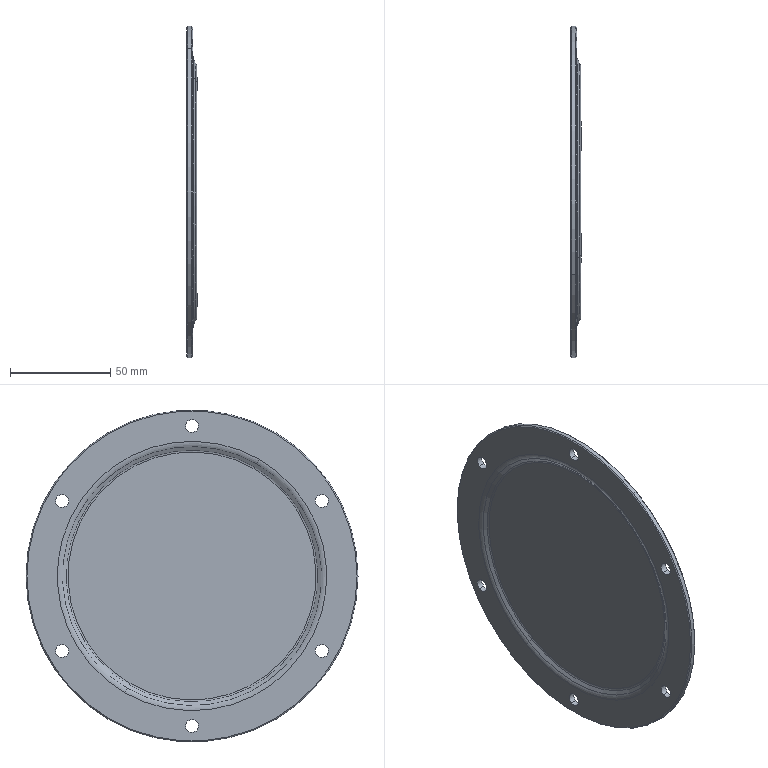Part | SolidWorks | features BaseBody 1 | 1 solid | 34 faces | box 5 x 166 x 166 mm | volume 64748 mm3 | cylinder 14 | cone 8 | torus 8 | plane 4 | commonest cylinder face diameters 6.5 x12 166 x2
STEP:
#1=CARTESIAN_POINT('',(330.,-41.5,71.88));
#2=VERTEX_POINT('',#1);
#3=CARTESIAN_POINT('',(330.,41.5,-71.88));
#4=VERTEX_POINT('',#3);
#5=CARTESIAN_POINT('',(330.,0.,0.));
#6=DIRECTION('',(-1.,0.,0.));
#7=DIRECTION('',(0.,-0.5,0.866));
#8=AXIS2_PLACEMENT_3D('',#5,#6,#7);
#9=CIRCLE('',#8,83.);
#10=EDGE_CURVE('',#2,#4,#9,.T.);
#11=ORIENTED_EDGE('',*,*,#10,.T.);
#12=CARTESIAN_POINT('',(328.,41.5,-71.88));
#13=VERTEX_POINT('',#12);
#14=CARTESIAN_POINT('',(330.,41.5,-71.88));
#15=DIRECTION('',(-1.,0.,0.));
#16=VECTOR('',#15,1000.);
#17=LINE('',#14,#16);
#18=EDGE_CURVE('',#4,#13,#17,.T.);
#19=ORIENTED_EDGE('',*,*,#18,.T.);
#20=CARTESIAN_POINT('',(328.,-41.5,71.88));
#21=VERTEX_POINT('',#20);
#22=CARTESIAN_POINT('',(328.,0.,0.));
#23=DIRECTION('',(1.,0.,0.));
#24=DIRECTION('',(0.,0.5,-0.866));
#25=AXIS2_PLACEMENT_3D('',#22,#23,#24);
#26=CIRCLE('',#25,83.);
#27=EDGE_CURVE('',#13,#21,#26,.T.);
#28=ORIENTED_EDGE('',*,*,#27,.T.);
#29=CARTESIAN_POINT('',(330.,-41.5,71.88));
#30=DIRECTION('',(-1.,0.,0.));
#31=VECTOR('',#30,1000.);
#32=LINE('',#29,#31);
#33=EDGE_CURVE('',#2,#21,#32,.T.);
#34=ORIENTED_EDGE('',*,*,#33,.F.);
#35=EDGE_LOOP('',(#11,#19,#28,#34));
#36=FACE_OUTER_BOUND('',#35,.T.);
#37=CARTESIAN_POINT('',(330.,0.,0.));
#38=DIRECTION('',(-1.,0.,0.));
#39=DIRECTION('',(0.,-0.5,0.866));
#40=AXIS2_PLACEMENT_3D('',#37,#38,#39);
#41=CYLINDRICAL_SURFACE('',#40,83.);
#42=ADVANCED_FACE('',(#36),#41,.T.);
#43=CARTESIAN_POINT('',(331.83,-32.25,55.859));
#44=VERTEX_POINT('',#43);
#45=CARTESIAN_POINT('',(331.83,32.25,-55.859));
#46=VERTEX_POINT('',#45);
#47=CARTESIAN_POINT('',(331.83,0.,0.));
#48=DIRECTION('',(-1.,0.,0.));
#49=DIRECTION('',(0.,0.5,-0.866));
#50=AXIS2_PLACEMENT_3D('',#47,#48,#49);
#51=CIRCLE('',#50,64.5);
#52=EDGE_CURVE('',#44,#46,#51,.T.);
#53=ORIENTED_EDGE('',*,*,#52,.T.);
#54=CARTESIAN_POINT('',(330.768,33.17,-57.452));
#55=VERTEX_POINT('',#54);
#56=CARTESIAN_POINT('',(368.069,0.866,-1.5));
#57=DIRECTION('',(-0.5,0.433,-0.75));
#58=VECTOR('',#57,1000.);
#59=LINE('',#56,#58);
#60=EDGE_CURVE('',#46,#55,#59,.T.);
#61=ORIENTED_EDGE('',*,*,#60,.T.);
#62=CARTESIAN_POINT('',(330.768,-33.17,57.452));
#63=VERTEX_POINT('',#62);
#64=CARTESIAN_POINT('',(330.768,0.,0.));
#65=DIRECTION('',(1.,0.,0.));
#66=DIRECTION('',(0.,0.5,-0.866));
#67=AXIS2_PLACEMENT_3D('',#64,#65,#66);
#68=CIRCLE('',#67,66.34);
#69=EDGE_CURVE('',#55,#63,#68,.T.);
#70=ORIENTED_EDGE('',*,*,#69,.T.);
#71=CARTESIAN_POINT('',(368.069,-0.866,1.5));
#72=DIRECTION('',(-0.5,-0.433,0.75));
#73=VECTOR('',#72,1000.);
#74=LINE('',#71,#73);
#75=EDGE_CURVE('',#44,#63,#74,.T.);
#76=ORIENTED_EDGE('',*,*,#75,.F.);
#77=EDGE_LOOP('',(#53,#61,#70,#76));
#78=FACE_OUTER_BOUND('',#77,.T.);
#79=CARTESIAN_POINT('',(368.069,0.,0.));
#80=DIRECTION('',(-1.,0.,0.));
#81=DIRECTION('',(0.,-0.5,0.866));
#82=AXIS2_PLACEMENT_3D('',#79,#80,#81);
#83=CONICAL_SURFACE('',#82,1.732,1.047);
#84=ADVANCED_FACE('',(#78),#83,.T.);
#85=CARTESIAN_POINT('',(329.232,-31.5,54.56));
#86=VERTEX_POINT('',#85);
#87=CARTESIAN_POINT('',(329.232,31.5,-54.56));
#88=VERTEX_POINT('',#87);
#89=CARTESIAN_POINT('',(329.232,0.,0.));
#90=DIRECTION('',(1.,0.,0.));
#91=DIRECTION('',(0.,0.5,-0.866));
#92=AXIS2_PLACEMENT_3D('',#89,#90,#91);
#93=CIRCLE('',#92,63.);
#94=EDGE_CURVE('',#86,#88,#93,.T.);
#95=ORIENTED_EDGE('',*,*,#94,.T.);
#96=CARTESIAN_POINT('',(328.17,32.42,-56.153));
#97=VERTEX_POINT('',#96);
#98=CARTESIAN_POINT('',(364.605,0.866,-1.5));
#99=DIRECTION('',(-0.5,0.433,-0.75));
#100=VECTOR('',#99,1000.);
#101=LINE('',#98,#100);
#102=EDGE_CURVE('',#88,#97,#101,.T.);
#103=ORIENTED_EDGE('',*,*,#102,.T.);
#104=CARTESIAN_POINT('',(328.17,-32.42,56.153));
#105=VERTEX_POINT('',#104);
#106=CARTESIAN_POINT('',(328.17,0.,0.));
#107=DIRECTION('',(-1.,0.,0.));
#108=DIRECTION('',(0.,0.5,-0.866));
#109=AXIS2_PLACEMENT_3D('',#106,#107,#108);
#110=CIRCLE('',#109,64.84);
#111=EDGE_CURVE('',#97,#105,#110,.T.);
#112=ORIENTED_EDGE('',*,*,#111,.T.);
#113=CARTESIAN_POINT('',(364.605,-0.866,1.5));
#114=DIRECTION('',(-0.5,-0.433,0.75));
#115=VECTOR('',#114,1000.);
#116=LINE('',#113,#115);
#117=EDGE_CURVE('',#86,#105,#116,.T.);
#118=ORIENTED_EDGE('',*,*,#117,.F.);
#119=EDGE_LOOP('',(#95,#103,#112,#118));
#120=FACE_OUTER_BOUND('',#119,.T.);
#121=CARTESIAN_POINT('',(364.605,0.,0.));
#122=DIRECTION('',(-1.,0.,0.));
#123=DIRECTION('',(0.,-0.5,0.866));
#124=AXIS2_PLACEMENT_3D('',#121,#122,#123);
#125=CONICAL_SURFACE('',#124,1.732,1.047);
#126=ADVANCED_FACE('',(#120),#125,.F.);
#127=ORIENTED_EDGE('',*,*,#52,.F.);
#128=CARTESIAN_POINT('',(332.5,-31.,53.694));
#129=VERTEX_POINT('',#128);
#130=CARTESIAN_POINT('',(327.5,-31.,53.694));
#131=DIRECTION('',(0.,0.866,0.5));
#132=DIRECTION('',(0.,-0.5,0.866));
#133=AXIS2_PLACEMENT_3D('',#130,#131,#132);
#134=CIRCLE('',#133,5.);
#135=EDGE_CURVE('',#44,#129,#134,.T.);
#136=ORIENTED_EDGE('',*,*,#135,.T.);
#137=CARTESIAN_POINT('',(332.5,31.,-53.694));
#138=VERTEX_POINT('',#137);
#139=CARTESIAN_POINT('',(332.5,0.,0.));
#140=DIRECTION('',(1.,0.,0.));
#141=DIRECTION('',(0.,-0.5,0.866));
#142=AXIS2_PLACEMENT_3D('',#139,#140,#141);
#143=CIRCLE('',#142,62.);
#144=EDGE_CURVE('',#138,#129,#143,.T.);
#145=ORIENTED_EDGE('',*,*,#144,.F.);
#146=CARTESIAN_POINT('',(327.5,31.,-53.694));
#147=DIRECTION('',(0.,-0.866,-0.5));
#148=DIRECTION('',(0.,0.5,-0.866));
#149=AXIS2_PLACEMENT_3D('',#146,#147,#148);
#150=CIRCLE('',#149,5.);
#151=EDGE_CURVE('',#46,#138,#150,.T.);
#152=ORIENTED_EDGE('',*,*,#151,.F.);
#153=EDGE_LOOP('',(#127,#136,#145,#152));
#154=FACE_OUTER_BOUND('',#153,.T.);
#155=CARTESIAN_POINT('',(327.5,0.,0.));
#156=DIRECTION('',(1.,0.,0.));
#157=DIRECTION('',(0.,0.5,-0.866));
#158=AXIS2_PLACEMENT_3D('',#155,#156,#157);
#159=TOROIDAL_SURFACE('',#158,62.,5.);
#160=ADVANCED_FACE('',(#154),#159,.T.);
#161=CARTESIAN_POINT('',(327.5,33.67,-58.318));
#162=VERTEX_POINT('',#161);
#163=CARTESIAN_POINT('',(327.5,-33.67,58.318));
#164=VERTEX_POINT('',#163);
#165=CARTESIAN_POINT('',(327.5,0.,0.));
#166=DIRECTION('',(1.,0.,0.));
#167=DIRECTION('',(0.,0.5,-0.866));
#168=AXIS2_PLACEMENT_3D('',#165,#166,#167);
#169=CIRCLE('',#168,67.34);
#170=EDGE_CURVE('',#162,#164,#169,.T.);
#171=ORIENTED_EDGE('',*,*,#170,.F.);
#172=CARTESIAN_POINT('',(332.5,33.67,-58.318));
#173=DIRECTION('',(0.,0.866,0.5));
#174=DIRECTION('',(0.,-0.5,0.866));
#175=AXIS2_PLACEMENT_3D('',#172,#173,#174);
#176=CIRCLE('',#175,5.);
#177=EDGE_CURVE('',#162,#97,#176,.T.);
#178=ORIENTED_EDGE('',*,*,#177,.T.);
#179=CARTESIAN_POINT('',(328.17,0.,0.));
#180=DIRECTION('',(-1.,0.,0.));
#181=DIRECTION('',(0.,0.5,-0.866));
#182=AXIS2_PLACEMENT_3D('',#179,#180,#181);
#183=CIRCLE('',#182,64.84);
#184=EDGE_CURVE('',#105,#97,#183,.T.);
#185=ORIENTED_EDGE('',*,*,#184,.F.);
#186=CARTESIAN_POINT('',(332.5,-33.67,58.318));
#187=DIRECTION('',(0.,-0.866,-0.5));
#188=DIRECTION('',(0.,0.5,-0.866));
#189=AXIS2_PLACEMENT_3D('',#186,#187,#188);
#190=CIRCLE('',#189,5.);
#191=EDGE_CURVE('',#164,#105,#190,.T.);
#192=ORIENTED_EDGE('',*,*,#191,.F.);
#193=EDGE_LOOP('',(#171,#178,#185,#192));
#194=FACE_OUTER_BOUND('',#193,.T.);
#195=CARTESIAN_POINT('',(332.5,0.,0.));
#196=DIRECTION('',(-1.,0.,0.));
#197=DIRECTION('',(0.,-0.5,0.866));
#198=AXIS2_PLACEMENT_3D('',#195,#196,#197);
#199=TOROIDAL_SURFACE('',#198,67.34,5.);
#200=ADVANCED_FACE('',(#194),#199,.T.);
#201=CARTESIAN_POINT('',(330.768,0.,0.));
#202=DIRECTION('',(1.,0.,0.));
#203=DIRECTION('',(0.,0.5,-0.866));
#204=AXIS2_PLACEMENT_3D('',#201,#202,#203);
#205=CIRCLE('',#204,66.34);
#206=EDGE_CURVE('',#63,#55,#205,.T.);
#207=ORIENTED_EDGE('',*,*,#206,.F.);
#208=CARTESIAN_POINT('',(330.5,-33.67,58.318));
#209=VERTEX_POINT('',#208);
#210=CARTESIAN_POINT('',(332.5,-33.67,58.318));
#211=DIRECTION('',(0.,0.866,0.5));
#212=DIRECTION('',(0.,-0.5,0.866));
#213=AXIS2_PLACEMENT_3D('',#210,#211,#212);
#214=CIRCLE('',#213,2.);
#215=EDGE_CURVE('',#63,#209,#214,.T.);
#216=ORIENTED_EDGE('',*,*,#215,.T.);
#217=CARTESIAN_POINT('',(330.5,33.67,-58.318));
#218=VERTEX_POINT('',#217);
#219=CARTESIAN_POINT('',(330.5,0.,0.));
#220=DIRECTION('',(-1.,0.,0.));
#221=DIRECTION('',(0.,-0.5,0.866));
#222=AXIS2_PLACEMENT_3D('',#219,#220,#221);
#223=CIRCLE('',#222,67.34);
#224=EDGE_CURVE('',#218,#209,#223,.T.);
#225=ORIENTED_EDGE('',*,*,#224,.F.);
#226=CARTESIAN_POINT('',(332.5,33.67,-58.318));
#227=DIRECTION('',(0.,-0.866,-0.5));
#228=DIRECTION('',(0.,0.5,-0.866));
#229=AXIS2_PLACEMENT_3D('',#226,#227,#228);
#230=CIRCLE('',#229,2.);
#231=EDGE_CURVE('',#55,#218,#230,.T.);
#232=ORIENTED_EDGE('',*,*,#231,.F.);
#233=EDGE_LOOP('',(#207,#216,#225,#232));
#234=FACE_OUTER_BOUND('',#233,.T.);
#235=CARTESIAN_POINT('',(332.5,0.,0.));
#236=DIRECTION('',(1.,0.,0.));
#237=DIRECTION('',(0.,0.5,-0.866));
#238=AXIS2_PLACEMENT_3D('',#235,#236,#237);
#239=TOROIDAL_SURFACE('',#238,67.34,2.);
#240=ADVANCED_FACE('',(#234),#239,.F.);
#241=CARTESIAN_POINT('',(329.5,31.,-53.694));
#242=VERTEX_POINT('',#241);
#243=CARTESIAN_POINT('',(329.5,-31.,53.694));
#244=VERTEX_POINT('',#243);
#245=CARTESIAN_POINT('',(329.5,0.,0.));
#246=DIRECTION('',(-1.,0.,0.));
#247=DIRECTION('',(0.,0.5,-0.866));
#248=AXIS2_PLACEMENT_3D('',#245,#246,#247);
#249=CIRCLE('',#248,62.);
#250=EDGE_CURVE('',#242,#244,#249,.T.);
#251=ORIENTED_EDGE('',*,*,#250,.F.);
#252=CARTESIAN_POINT('',(327.5,31.,-53.694));
#253=DIRECTION('',(0.,0.866,0.5));
#254=DIRECTION('',(0.,-0.5,0.866));
#255=AXIS2_PLACEMENT_3D('',#252,#253,#254);
#256=CIRCLE('',#255,2.);
#257=EDGE_CURVE('',#242,#88,#256,.T.);
#258=ORIENTED_EDGE('',*,*,#257,.T.);
#259=ORIENTED_EDGE('',*,*,#94,.F.);
#260=CARTESIAN_POINT('',(327.5,-31.,53.694));
#261=DIRECTION('',(0.,-0.866,-0.5));
#262=DIRECTION('',(0.,0.5,-0.866));
#263=AXIS2_PLACEMENT_3D('',#260,#261,#262);
#264=CIRCLE('',#263,2.);
#265=EDGE_CURVE('',#244,#86,#264,.T.);
#266=ORIENTED_EDGE('',*,*,#265,.F.);
#267=EDGE_LOOP('',(#251,#258,#259,#266));
#268=FACE_OUTER_BOUND('',#267,.T.);
#269=CARTESIAN_POINT('',(327.5,0.,0.));
#270=DIRECTION('',(-1.,0.,0.));
#271=DIRECTION('',(0.,-0.5,0.866));
#272=AXIS2_PLACEMENT_3D('',#269,#270,#271);
#273=TOROIDAL_SURFACE('',#272,62.,2.);
#274=ADVANCED_FACE('',(#268),#273,.F.);
#275=CARTESIAN_POINT('',(330.5,41.25,-71.447));
#276=VERTEX_POINT('',#275);
#277=CARTESIAN_POINT('',(330.5,-41.25,71.447));
#278=VERTEX_POINT('',#277);
#279=CARTESIAN_POINT('',(330.5,0.,0.));
#280=DIRECTION('',(1.,0.,0.));
#281=DIRECTION('',(0.,-0.5,0.866));
#282=AXIS2_PLACEMENT_3D('',#279,#280,#281);
#283=CIRCLE('',#282,82.5);
#284=EDGE_CURVE('',#276,#278,#283,.T.);
#285=ORIENTED_EDGE('',*,*,#284,.F.);
#286=CARTESIAN_POINT('',(412.,0.5,-0.866));
#287=DIRECTION('',(-0.7071,0.3536,-0.6124));
#288=VECTOR('',#287,1000.);
#289=LINE('',#286,#288);
#290=EDGE_CURVE('',#276,#4,#289,.T.);
#291=ORIENTED_EDGE('',*,*,#290,.T.);
#292=ORIENTED_EDGE('',*,*,#10,.F.);
#293=CARTESIAN_POINT('',(412.,-0.5,0.866));
#294=DIRECTION('',(-0.7071,-0.3536,0.6124));
#295=VECTOR('',#294,1000.);
#296=LINE('',#293,#295);
#297=EDGE_CURVE('',#278,#2,#296,.T.);
#298=ORIENTED_EDGE('',*,*,#297,.F.);
#299=EDGE_LOOP('',(#285,#291,#292,#298));
#300=FACE_OUTER_BOUND('',#299,.T.);
#301=CARTESIAN_POINT('',(412.,0.,0.));
#302=DIRECTION('',(-1.,0.,0.));
#303=DIRECTION('',(0.,-0.5,0.866));
#304=AXIS2_PLACEMENT_3D('',#301,#302,#303);
#305=CONICAL_SURFACE('',#304,1.,0.7854);
#306=ADVANCED_FACE('',(#300),#305,.T.);
#307=CARTESIAN_POINT('',(327.5,-41.25,71.447));
#308=VERTEX_POINT('',#307);
#309=CARTESIAN_POINT('',(327.5,41.25,-71.447));
#310=VERTEX_POINT('',#309);
#311=CARTESIAN_POINT('',(327.5,0.,0.));
#312=DIRECTION('',(-1.,0.,0.));
#313=DIRECTION('',(0.,0.5,-0.866));
#314=AXIS2_PLACEMENT_3D('',#311,#312,#313);
#315=CIRCLE('',#314,82.5);
#316=EDGE_CURVE('',#308,#310,#315,.T.);
#317=ORIENTED_EDGE('',*,*,#316,.F.);
#318=CARTESIAN_POINT('',(246.,-0.5,0.866));
#319=DIRECTION('',(0.7071,-0.3536,0.6124));
#320=VECTOR('',#319,1000.);
#321=LINE('',#318,#320);
#322=EDGE_CURVE('',#308,#21,#321,.T.);
#323=ORIENTED_EDGE('',*,*,#322,.T.);
#324=ORIENTED_EDGE('',*,*,#27,.F.);
#325=CARTESIAN_POINT('',(246.,0.5,-0.866));
#326=DIRECTION('',(0.7071,0.3536,-0.6124));
#327=VECTOR('',#326,1000.);
#328=LINE('',#325,#327);
#329=EDGE_CURVE('',#310,#13,#328,.T.);
#330=ORIENTED_EDGE('',*,*,#329,.F.);
#331=EDGE_LOOP('',(#317,#323,#324,#330));
#332=FACE_OUTER_BOUND('',#331,.T.);
#333=CARTESIAN_POINT('',(246.,0.,0.));
#334=DIRECTION('',(1.,0.,0.));
#335=DIRECTION('',(0.,0.5,-0.866));
#336=AXIS2_PLACEMENT_3D('',#333,#334,#335);
#337=CONICAL_SURFACE('',#336,1.,0.7854);
#338=ADVANCED_FACE('',(#332),#337,.T.);
#339=CARTESIAN_POINT('',(330.5,-63.327,34.685));
#340=VERTEX_POINT('',#339);
#341=CARTESIAN_POINT('',(330.5,-66.577,40.315));
#342=VERTEX_POINT('',#341);
#343=CARTESIAN_POINT('',(330.5,-64.952,37.5));
#344=DIRECTION('',(-1.,0.,0.));
#345=DIRECTION('',(0.,0.5,-0.866));
#346=AXIS2_PLACEMENT_3D('',#343,#344,#345);
#347=CIRCLE('',#346,3.25);
#348=EDGE_CURVE('',#340,#342,#347,.T.);
#349=ORIENTED_EDGE('',*,*,#348,.F.);
#350=CARTESIAN_POINT('',(327.5,-63.327,34.685));
#351=VERTEX_POINT('',#350);
#352=CARTESIAN_POINT('',(330.5,-63.327,34.685));
#353=DIRECTION('',(-1.,0.,0.));
#354=VECTOR('',#353,1000.);
#355=LINE('',#352,#354);
#356=EDGE_CURVE('',#340,#351,#355,.T.);
#357=ORIENTED_EDGE('',*,*,#356,.T.);
#358=CARTESIAN_POINT('',(327.5,-66.577,40.315));
#359=VERTEX_POINT('',#358);
#360=CARTESIAN_POINT('',(327.5,-64.952,37.5));
#361=DIRECTION('',(1.,0.,0.));
#362=DIRECTION('',(0.,0.5,-0.866));
#363=AXIS2_PLACEMENT_3D('',#360,#361,#362);
#364=CIRCLE('',#363,3.25);
#365=EDGE_CURVE('',#359,#351,#364,.T.);
#366=ORIENTED_EDGE('',*,*,#365,.F.);
#367=CARTESIAN_POINT('',(330.5,-66.577,40.315));
#368=DIRECTION('',(-1.,0.,0.));
#369=VECTOR('',#368,1000.);
#370=LINE('',#367,#369);
#371=EDGE_CURVE('',#342,#359,#370,.T.);
#372=ORIENTED_EDGE('',*,*,#371,.F.);
#373=EDGE_LOOP('',(#349,#357,#366,#372));
#374=FACE_OUTER_BOUND('',#373,.T.);
#375=CARTESIAN_POINT('',(330.5,-64.952,37.5));
#376=DIRECTION('',(-1.,0.,0.));
#377=DIRECTION('',(0.,-0.5,0.866));
#378=AXIS2_PLACEMENT_3D('',#375,#376,#377);
#379=CYLINDRICAL_SURFACE('',#378,3.25);
#380=ADVANCED_FACE('',(#374),#379,.F.);
#381=CARTESIAN_POINT('',(330.5,1.625,72.185));
#382=VERTEX_POINT('',#381);
#383=CARTESIAN_POINT('',(330.5,-1.625,77.815));
#384=VERTEX_POINT('',#383);
#385=CARTESIAN_POINT('',(330.5,0.,75.));
#386=DIRECTION('',(-1.,0.,0.));
#387=DIRECTION('',(0.,0.5,-0.866));
#388=AXIS2_PLACEMENT_3D('',#385,#386,#387);
#389=CIRCLE('',#388,3.25);
#390=EDGE_CURVE('',#382,#384,#389,.T.);
#391=ORIENTED_EDGE('',*,*,#390,.F.);
#392=CARTESIAN_POINT('',(327.5,1.625,72.185));
#393=VERTEX_POINT('',#392);
#394=CARTESIAN_POINT('',(330.5,1.625,72.185));
#395=DIRECTION('',(-1.,0.,0.));
#396=VECTOR('',#395,1000.);
#397=LINE('',#394,#396);
#398=EDGE_CURVE('',#382,#393,#397,.T.);
#399=ORIENTED_EDGE('',*,*,#398,.T.);
#400=CARTESIAN_POINT('',(327.5,-1.625,77.815));
#401=VERTEX_POINT('',#400);
#402=CARTESIAN_POINT('',(327.5,0.,75.));
#403=DIRECTION('',(1.,0.,0.));
#404=DIRECTION('',(0.,0.5,-0.866));
#405=AXIS2_PLACEMENT_3D('',#402,#403,#404);
#406=CIRCLE('',#405,3.25);
#407=EDGE_CURVE('',#401,#393,#406,.T.);
#408=ORIENTED_EDGE('',*,*,#407,.F.);
#409=CARTESIAN_POINT('',(330.5,-1.625,77.815));
#410=DIRECTION('',(-1.,0.,0.));
#411=VECTOR('',#410,1000.);
#412=LINE('',#409,#411);
#413=EDGE_CURVE('',#384,#401,#412,.T.);
#414=ORIENTED_EDGE('',*,*,#413,.F.);
#415=EDGE_LOOP('',(#391,#399,#408,#414));
#416=FACE_OUTER_BOUND('',#415,.T.);
#417=CARTESIAN_POINT('',(330.5,0.,75.));
#418=DIRECTION('',(-1.,0.,0.));
#419=DIRECTION('',(0.,-0.5,0.866));
#420=AXIS2_PLACEMENT_3D('',#417,#418,#419);
#421=CYLINDRICAL_SURFACE('',#420,3.25);
#422=ADVANCED_FACE('',(#416),#421,.F.);
#423=CARTESIAN_POINT('',(330.5,66.577,34.685));
#424=VERTEX_POINT('',#423);
#425=CARTESIAN_POINT('',(330.5,63.327,40.315));
#426=VERTEX_POINT('',#425);
#427=CARTESIAN_POINT('',(330.5,64.952,37.5));
#428=DIRECTION('',(-1.,0.,0.));
#429=DIRECTION('',(0.,0.5,-0.866));
#430=AXIS2_PLACEMENT_3D('',#427,#428,#429);
#431=CIRCLE('',#430,3.25);
#432=EDGE_CURVE('',#424,#426,#431,.T.);
#433=ORIENTED_EDGE('',*,*,#432,.F.);
#434=CARTESIAN_POINT('',(327.5,66.577,34.685));
#435=VERTEX_POINT('',#434);
#436=CARTESIAN_POINT('',(330.5,66.577,34.685));
#437=DIRECTION('',(-1.,0.,0.));
#438=VECTOR('',#437,1000.);
#439=LINE('',#436,#438);
#440=EDGE_CURVE('',#424,#435,#439,.T.);
#441=ORIENTED_EDGE('',*,*,#440,.T.);
#442=CARTESIAN_POINT('',(327.5,63.327,40.315));
#443=VERTEX_POINT('',#442);
#444=CARTESIAN_POINT('',(327.5,64.952,37.5));
#445=DIRECTION('',(1.,0.,0.));
#446=DIRECTION('',(0.,0.5,-0.866));
#447=AXIS2_PLACEMENT_3D('',#444,#445,#446);
#448=CIRCLE('',#447,3.25);
#449=EDGE_CURVE('',#443,#435,#448,.T.);
#450=ORIENTED_EDGE('',*,*,#449,.F.);
#451=CARTESIAN_POINT('',(330.5,63.327,40.315));
#452=DIRECTION('',(-1.,0.,0.));
#453=VECTOR('',#452,1000.);
#454=LINE('',#451,#453);
#455=EDGE_CURVE('',#426,#443,#454,.T.);
#456=ORIENTED_EDGE('',*,*,#455,.F.);
#457=EDGE_LOOP('',(#433,#441,#450,#456));
#458=FACE_OUTER_BOUND('',#457,.T.);
#459=CARTESIAN_POINT('',(330.5,64.952,37.5));
#460=DIRECTION('',(-1.,0.,0.));
#461=DIRECTION('',(0.,-0.5,0.866));
#462=AXIS2_PLACEMENT_3D('',#459,#460,#461);
#463=CYLINDRICAL_SURFACE('',#462,3.25);
#464=ADVANCED_FACE('',(#458),#463,.F.);
#465=CARTESIAN_POINT('',(330.5,66.577,-40.315));
#466=VERTEX_POINT('',#465);
#467=CARTESIAN_POINT('',(330.5,63.327,-34.685));
#468=VERTEX_POINT('',#467);
#469=CARTESIAN_POINT('',(330.5,64.952,-37.5));
#470=DIRECTION('',(-1.,0.,0.));
#471=DIRECTION('',(0.,0.5,-0.866));
#472=AXIS2_PLACEMENT_3D('',#469,#470,#471);
#473=CIRCLE('',#472,3.25);
#474=EDGE_CURVE('',#466,#468,#473,.T.);
#475=ORIENTED_EDGE('',*,*,#474,.F.);
#476=CARTESIAN_POINT('',(327.5,66.577,-40.315));
#477=VERTEX_POINT('',#476);
#478=CARTESIAN_POINT('',(330.5,66.577,-40.315));
#479=DIRECTION('',(-1.,0.,0.));
#480=VECTOR('',#479,1000.);
#481=LINE('',#478,#480);
#482=EDGE_CURVE('',#466,#477,#481,.T.);
#483=ORIENTED_EDGE('',*,*,#482,.T.);
#484=CARTESIAN_POINT('',(327.5,63.327,-34.685));
#485=VERTEX_POINT('',#484);
#486=CARTESIAN_POINT('',(327.5,64.952,-37.5));
#487=DIRECTION('',(1.,0.,0.));
#488=DIRECTION('',(0.,0.5,-0.866));
#489=AXIS2_PLACEMENT_3D('',#486,#487,#488);
#490=CIRCLE('',#489,3.25);
#491=EDGE_CURVE('',#485,#477,#490,.T.);
#492=ORIENTED_EDGE('',*,*,#491,.F.);
#493=CARTESIAN_POINT('',(330.5,63.327,-34.685));
#494=DIRECTION('',(-1.,0.,0.));
#495=VECTOR('',#494,1000.);
#496=LINE('',#493,#495);
#497=EDGE_CURVE('',#468,#485,#496,.T.);
#498=ORIENTED_EDGE('',*,*,#497,.F.);
#499=EDGE_LOOP('',(#475,#483,#492,#498));
#500=FACE_OUTER_BOUND('',#499,.T.);
#501=CARTESIAN_POINT('',(330.5,64.952,-37.5));
#502=DIRECTION('',(-1.,0.,0.));
#503=DIRECTION('',(0.,-0.5,0.866));
#504=AXIS2_PLACEMENT_3D('',#501,#502,#503);
#505=CYLINDRICAL_SURFACE('',#504,3.25);
#506=ADVANCED_FACE('',(#500),#505,.F.);
#507=CARTESIAN_POINT('',(330.5,1.625,-77.815));
#508=VERTEX_POINT('',#507);
#509=CARTESIAN_POINT('',(330.5,-1.625,-72.185));
#510=VERTEX_POINT('',#509);
#511=CARTESIAN_POINT('',(330.5,0.,-75.));
#512=DIRECTION('',(-1.,0.,0.));
#513=DIRECTION('',(0.,0.5,-0.866));
#514=AXIS2_PLACEMENT_3D('',#511,#512,#513);
#515=CIRCLE('',#514,3.25);
#516=EDGE_CURVE('',#508,#510,#515,.T.);
#517=ORIENTED_EDGE('',*,*,#516,.F.);
#518=CARTESIAN_POINT('',(327.5,1.625,-77.815));
#519=VERTEX_POINT('',#518);
#520=CARTESIAN_POINT('',(330.5,1.625,-77.815));
#521=DIRECTION('',(-1.,0.,0.));
#522=VECTOR('',#521,1000.);
#523=LINE('',#520,#522);
#524=EDGE_CURVE('',#508,#519,#523,.T.);
#525=ORIENTED_EDGE('',*,*,#524,.T.);
#526=CARTESIAN_POINT('',(327.5,-1.625,-72.185));
#527=VERTEX_POINT('',#526);
#528=CARTESIAN_POINT('',(327.5,0.,-75.));
#529=DIRECTION('',(1.,0.,0.));
#530=DIRECTION('',(0.,0.5,-0.866));
#531=AXIS2_PLACEMENT_3D('',#528,#529,#530);
#532=CIRCLE('',#531,3.25);
#533=EDGE_CURVE('',#527,#519,#532,.T.);
#534=ORIENTED_EDGE('',*,*,#533,.F.);
#535=CARTESIAN_POINT('',(330.5,-1.625,-72.185));
#536=DIRECTION('',(-1.,0.,0.));
#537=VECTOR('',#536,1000.);
#538=LINE('',#535,#537);
#539=EDGE_CURVE('',#510,#527,#538,.T.);
#540=ORIENTED_EDGE('',*,*,#539,.F.);
#541=EDGE_LOOP('',(#517,#525,#534,#540));
#542=FACE_OUTER_BOUND('',#541,.T.);
#543=CARTESIAN_POINT('',(330.5,0.,-75.));
#544=DIRECTION('',(-1.,0.,0.));
#545=DIRECTION('',(0.,-0.5,0.866));
#546=AXIS2_PLACEMENT_3D('',#543,#544,#545);
#547=CYLINDRICAL_SURFACE('',#546,3.25);
#548=ADVANCED_FACE('',(#542),#547,.F.);
#549=CARTESIAN_POINT('',(330.5,-63.327,-40.315));
#550=VERTEX_POINT('',#549);
#551=CARTESIAN_POINT('',(330.5,-66.577,-34.685));
#552=VERTEX_POINT('',#551);
#553=CARTESIAN_POINT('',(330.5,-64.952,-37.5));
#554=DIRECTION('',(-1.,0.,0.));
#555=DIRECTION('',(0.,0.5,-0.866));
#556=AXIS2_PLACEMENT_3D('',#553,#554,#555);
#557=CIRCLE('',#556,3.25);
#558=EDGE_CURVE('',#550,#552,#557,.T.);
#559=ORIENTED_EDGE('',*,*,#558,.F.);
#560=CARTESIAN_POINT('',(327.5,-63.327,-40.315));
#561=VERTEX_POINT('',#560);
#562=CARTESIAN_POINT('',(330.5,-63.327,-40.315));
#563=DIRECTION('',(-1.,0.,0.));
#564=VECTOR('',#563,1000.);
#565=LINE('',#562,#564);
#566=EDGE_CURVE('',#550,#561,#565,.T.);
#567=ORIENTED_EDGE('',*,*,#566,.T.);
#568=CARTESIAN_POINT('',(327.5,-66.577,-34.685));
#569=VERTEX_POINT('',#568);
#570=CARTESIAN_POINT('',(327.5,-64.952,-37.5));
#571=DIRECTION('',(1.,0.,0.));
#572=DIRECTION('',(0.,0.5,-0.866));
#573=AXIS2_PLACEMENT_3D('',#570,#571,#572);
#574=CIRCLE('',#573,3.25);
#575=EDGE_CURVE('',#569,#561,#574,.T.);
#576=ORIENTED_EDGE('',*,*,#575,.F.);
#577=CARTESIAN_POINT('',(330.5,-66.577,-34.685));
#578=DIRECTION('',(-1.,0.,0.));
#579=VECTOR('',#578,1000.);
#580=LINE('',#577,#579);
#581=EDGE_CURVE('',#552,#569,#580,.T.);
#582=ORIENTED_EDGE('',*,*,#581,.F.);
#583=EDGE_LOOP('',(#559,#567,#576,#582));
#584=FACE_OUTER_BOUND('',#583,.T.);
#585=CARTESIAN_POINT('',(330.5,-64.952,-37.5));
#586=DIRECTION('',(-1.,0.,0.));
#587=DIRECTION('',(0.,-0.5,0.866));
#588=AXIS2_PLACEMENT_3D('',#585,#586,#587);
#589=CYLINDRICAL_SURFACE('',#588,3.25);
#590=ADVANCED_FACE('',(#584),#589,.F.);
#591=ORIENTED_EDGE('',*,*,#566,.F.);
#592=CARTESIAN_POINT('',(330.5,-64.952,-37.5));
#593=DIRECTION('',(-1.,0.,0.));
#594=DIRECTION('',(0.,0.5,-0.866));
#595=AXIS2_PLACEMENT_3D('',#592,#593,#594);
#596=CIRCLE('',#595,3.25);
#597=EDGE_CURVE('',#552,#550,#596,.T.);
#598=ORIENTED_EDGE('',*,*,#597,.F.);
#599=ORIENTED_EDGE('',*,*,#581,.T.);
#600=CARTESIAN_POINT('',(327.5,-64.952,-37.5));
#601=DIRECTION('',(1.,0.,0.));
#602=DIRECTION('',(0.,0.5,-0.866));
#603=AXIS2_PLACEMENT_3D('',#600,#601,#602);
#604=CIRCLE('',#603,3.25);
#605=EDGE_CURVE('',#561,#569,#604,.T.);
#606=ORIENTED_EDGE('',*,*,#605,.F.);
#607=EDGE_LOOP('',(#591,#598,#599,#606));
#608=FACE_OUTER_BOUND('',#607,.T.);
#609=CARTESIAN_POINT('',(330.5,-64.952,-37.5));
#610=DIRECTION('',(-1.,0.,0.));
#611=DIRECTION('',(0.,-0.5,0.866));
#612=AXIS2_PLACEMENT_3D('',#609,#610,#611);
#613=CYLINDRICAL_SURFACE('',#612,3.25);
#614=ADVANCED_FACE('',(#608),#613,.F.);
#615=ORIENTED_EDGE('',*,*,#524,.F.);
#616=CARTESIAN_POINT('',(330.5,0.,-75.));
#617=DIRECTION('',(-1.,0.,0.));
#618=DIRECTION('',(0.,0.5,-0.866));
#619=AXIS2_PLACEMENT_3D('',#616,#617,#618);
#620=CIRCLE('',#619,3.25);
#621=EDGE_CURVE('',#510,#508,#620,.T.);
#622=ORIENTED_EDGE('',*,*,#621,.F.);
#623=ORIENTED_EDGE('',*,*,#539,.T.);
#624=CARTESIAN_POINT('',(327.5,0.,-75.));
#625=DIRECTION('',(1.,0.,0.));
#626=DIRECTION('',(0.,0.5,-0.866));
#627=AXIS2_PLACEMENT_3D('',#624,#625,#626);
#628=CIRCLE('',#627,3.25);
#629=EDGE_CURVE('',#519,#527,#628,.T.);
#630=ORIENTED_EDGE('',*,*,#629,.F.);
#631=EDGE_LOOP('',(#615,#622,#623,#630));
#632=FACE_OUTER_BOUND('',#631,.T.);
#633=CARTESIAN_POINT('',(330.5,0.,-75.));
#634=DIRECTION('',(-1.,0.,0.));
#635=DIRECTION('',(0.,-0.5,0.866));
#636=AXIS2_PLACEMENT_3D('',#633,#634,#635);
#637=CYLINDRICAL_SURFACE('',#636,3.25);
#638=ADVANCED_FACE('',(#632),#637,.F.);
#639=ORIENTED_EDGE('',*,*,#482,.F.);
#640=CARTESIAN_POINT('',(330.5,64.952,-37.5));
#641=DIRECTION('',(-1.,0.,0.));
#642=DIRECTION('',(0.,0.5,-0.866));
#643=AXIS2_PLACEMENT_3D('',#640,#641,#642);
#644=CIRCLE('',#643,3.25);
#645=EDGE_CURVE('',#468,#466,#644,.T.);
#646=ORIENTED_EDGE('',*,*,#645,.F.);
#647=ORIENTED_EDGE('',*,*,#497,.T.);
#648=CARTESIAN_POINT('',(327.5,64.952,-37.5));
#649=DIRECTION('',(1.,0.,0.));
#650=DIRECTION('',(0.,0.5,-0.866));
#651=AXIS2_PLACEMENT_3D('',#648,#649,#650);
#652=CIRCLE('',#651,3.25);
#653=EDGE_CURVE('',#477,#485,#652,.T.);
#654=ORIENTED_EDGE('',*,*,#653,.F.);
#655=EDGE_LOOP('',(#639,#646,#647,#654));
#656=FACE_OUTER_BOUND('',#655,.T.);
#657=CARTESIAN_POINT('',(330.5,64.952,-37.5));
#658=DIRECTION('',(-1.,0.,0.));
#659=DIRECTION('',(0.,-0.5,0.866));
#660=AXIS2_PLACEMENT_3D('',#657,#658,#659);
#661=CYLINDRICAL_SURFACE('',#660,3.25);
#662=ADVANCED_FACE('',(#656),#661,.F.);
#663=ORIENTED_EDGE('',*,*,#440,.F.);
#664=CARTESIAN_POINT('',(330.5,64.952,37.5));
#665=DIRECTION('',(-1.,0.,0.));
#666=DIRECTION('',(0.,0.5,-0.866));
#667=AXIS2_PLACEMENT_3D('',#664,#665,#666);
#668=CIRCLE('',#667,3.25);
#669=EDGE_CURVE('',#426,#424,#668,.T.);
#670=ORIENTED_EDGE('',*,*,#669,.F.);
#671=ORIENTED_EDGE('',*,*,#455,.T.);
#672=CARTESIAN_POINT('',(327.5,64.952,37.5));
#673=DIRECTION('',(1.,0.,0.));
#674=DIRECTION('',(0.,0.5,-0.866));
#675=AXIS2_PLACEMENT_3D('',#672,#673,#674);
#676=CIRCLE('',#675,3.25);
#677=EDGE_CURVE('',#435,#443,#676,.T.);
#678=ORIENTED_EDGE('',*,*,#677,.F.);
#679=EDGE_LOOP('',(#663,#670,#671,#678));
#680=FACE_OUTER_BOUND('',#679,.T.);
#681=CARTESIAN_POINT('',(330.5,64.952,37.5));
#682=DIRECTION('',(-1.,0.,0.));
#683=DIRECTION('',(0.,-0.5,0.866));
#684=AXIS2_PLACEMENT_3D('',#681,#682,#683);
#685=CYLINDRICAL_SURFACE('',#684,3.25);
#686=ADVANCED_FACE('',(#680),#685,.F.);
#687=ORIENTED_EDGE('',*,*,#398,.F.);
#688=CARTESIAN_POINT('',(330.5,0.,75.));
#689=DIRECTION('',(-1.,0.,0.));
#690=DIRECTION('',(0.,0.5,-0.866));
#691=AXIS2_PLACEMENT_3D('',#688,#689,#690);
#692=CIRCLE('',#691,3.25);
#693=EDGE_CURVE('',#384,#382,#692,.T.);
#694=ORIENTED_EDGE('',*,*,#693,.F.);
#695=ORIENTED_EDGE('',*,*,#413,.T.);
#696=CARTESIAN_POINT('',(327.5,0.,75.));
#697=DIRECTION('',(1.,0.,0.));
#698=DIRECTION('',(0.,0.5,-0.866));
#699=AXIS2_PLACEMENT_3D('',#696,#697,#698);
#700=CIRCLE('',#699,3.25);
#701=EDGE_CURVE('',#393,#401,#700,.T.);
#702=ORIENTED_EDGE('',*,*,#701,.F.);
#703=EDGE_LOOP('',(#687,#694,#695,#702));
#704=FACE_OUTER_BOUND('',#703,.T.);
#705=CARTESIAN_POINT('',(330.5,0.,75.));
#706=DIRECTION('',(-1.,0.,0.));
#707=DIRECTION('',(0.,-0.5,0.866));
#708=AXIS2_PLACEMENT_3D('',#705,#706,#707);
#709=CYLINDRICAL_SURFACE('',#708,3.25);
#710=ADVANCED_FACE('',(#704),#709,.F.);
#711=ORIENTED_EDGE('',*,*,#356,.F.);
#712=CARTESIAN_POINT('',(330.5,-64.952,37.5));
#713=DIRECTION('',(-1.,0.,0.));
#714=DIRECTION('',(0.,0.5,-0.866));
#715=AXIS2_PLACEMENT_3D('',#712,#713,#714);
#716=CIRCLE('',#715,3.25);
#717=EDGE_CURVE('',#342,#340,#716,.T.);
#718=ORIENTED_EDGE('',*,*,#717,.F.);
#719=ORIENTED_EDGE('',*,*,#371,.T.);
#720=CARTESIAN_POINT('',(327.5,-64.952,37.5));
#721=DIRECTION('',(1.,0.,0.));
#722=DIRECTION('',(0.,0.5,-0.866));
#723=AXIS2_PLACEMENT_3D('',#720,#721,#722);
#724=CIRCLE('',#723,3.25);
#725=EDGE_CURVE('',#351,#359,#724,.T.);
#726=ORIENTED_EDGE('',*,*,#725,.F.);
#727=EDGE_LOOP('',(#711,#718,#719,#726));
#728=FACE_OUTER_BOUND('',#727,.T.);
#729=CARTESIAN_POINT('',(330.5,-64.952,37.5));
#730=DIRECTION('',(-1.,0.,0.));
#731=DIRECTION('',(0.,-0.5,0.866));
#732=AXIS2_PLACEMENT_3D('',#729,#730,#731);
#733=CYLINDRICAL_SURFACE('',#732,3.25);
#734=ADVANCED_FACE('',(#728),#733,.F.);
#735=ORIENTED_EDGE('',*,*,#322,.F.);
#736=CARTESIAN_POINT('',(327.5,0.,0.));
#737=DIRECTION('',(-1.,0.,0.));
#738=DIRECTION('',(0.,0.5,-0.866));
#739=AXIS2_PLACEMENT_3D('',#736,#737,#738);
#740=CIRCLE('',#739,82.5);
#741=EDGE_CURVE('',#310,#308,#740,.T.);
#742=ORIENTED_EDGE('',*,*,#741,.F.);
#743=ORIENTED_EDGE('',*,*,#329,.T.);
#744=CARTESIAN_POINT('',(328.,0.,0.));
#745=DIRECTION('',(1.,0.,0.));
#746=DIRECTION('',(0.,0.5,-0.866));
#747=AXIS2_PLACEMENT_3D('',#744,#745,#746);
#748=CIRCLE('',#747,83.);
#749=EDGE_CURVE('',#21,#13,#748,.T.);
#750=ORIENTED_EDGE('',*,*,#749,.F.);
#751=EDGE_LOOP('',(#735,#742,#743,#750));
#752=FACE_OUTER_BOUND('',#751,.T.);
#753=CARTESIAN_POINT('',(246.,0.,0.));
#754=DIRECTION('',(1.,0.,0.));
#755=DIRECTION('',(0.,0.5,-0.866));
#756=AXIS2_PLACEMENT_3D('',#753,#754,#755);
#757=CONICAL_SURFACE('',#756,1.,0.7854);
#758=ADVANCED_FACE('',(#752),#757,.T.);
#759=ORIENTED_EDGE('',*,*,#290,.F.);
#760=CARTESIAN_POINT('',(330.5,0.,0.));
#761=DIRECTION('',(1.,0.,0.));
#762=DIRECTION('',(0.,-0.5,0.866));
#763=AXIS2_PLACEMENT_3D('',#760,#761,#762);
#764=CIRCLE('',#763,82.5);
#765=EDGE_CURVE('',#278,#276,#764,.T.);
#766=ORIENTED_EDGE('',*,*,#765,.F.);
#767=ORIENTED_EDGE('',*,*,#297,.T.);
#768=CARTESIAN_POINT('',(330.,0.,0.));
#769=DIRECTION('',(-1.,0.,0.));
#770=DIRECTION('',(0.,-0.5,0.866));
#771=AXIS2_PLACEMENT_3D('',#768,#769,#770);
#772=CIRCLE('',#771,83.);
#773=EDGE_CURVE('',#4,#2,#772,.T.);
#774=ORIENTED_EDGE('',*,*,#773,.F.);
#775=EDGE_LOOP('',(#759,#766,#767,#774));
#776=FACE_OUTER_BOUND('',#775,.T.);
#777=CARTESIAN_POINT('',(412.,0.,0.));
#778=DIRECTION('',(-1.,0.,0.));
#779=DIRECTION('',(0.,-0.5,0.866));
#780=AXIS2_PLACEMENT_3D('',#777,#778,#779);
#781=CONICAL_SURFACE('',#780,1.,0.7854);
#782=ADVANCED_FACE('',(#776),#781,.T.);
#783=ORIENTED_EDGE('',*,*,#257,.F.);
#784=CARTESIAN_POINT('',(329.5,0.,0.));
#785=DIRECTION('',(-1.,0.,0.));
#786=DIRECTION('',(0.,0.5,-0.866));
#787=AXIS2_PLACEMENT_3D('',#784,#785,#786);
#788=CIRCLE('',#787,62.);
#789=EDGE_CURVE('',#244,#242,#788,.T.);
#790=ORIENTED_EDGE('',*,*,#789,.F.);
#791=ORIENTED_EDGE('',*,*,#265,.T.);
#792=CARTESIAN_POINT('',(329.232,0.,0.));
#793=DIRECTION('',(1.,0.,0.));
#794=DIRECTION('',(0.,0.5,-0.866));
#795=AXIS2_PLACEMENT_3D('',#792,#793,#794);
#796=CIRCLE('',#795,63.);
#797=EDGE_CURVE('',#88,#86,#796,.T.);
#798=ORIENTED_EDGE('',*,*,#797,.F.);
#799=EDGE_LOOP('',(#783,#790,#791,#798));
#800=FACE_OUTER_BOUND('',#799,.T.);
#801=CARTESIAN_POINT('',(327.5,0.,0.));
#802=DIRECTION('',(-1.,0.,0.));
#803=DIRECTION('',(0.,-0.5,0.866));
#804=AXIS2_PLACEMENT_3D('',#801,#802,#803);
#805=TOROIDAL_SURFACE('',#804,62.,2.);
#806=ADVANCED_FACE('',(#800),#805,.F.);
#807=ORIENTED_EDGE('',*,*,#215,.F.);
#808=ORIENTED_EDGE('',*,*,#69,.F.);
#809=ORIENTED_EDGE('',*,*,#231,.T.);
#810=CARTESIAN_POINT('',(330.5,0.,0.));
#811=DIRECTION('',(-1.,0.,0.));
#812=DIRECTION('',(0.,-0.5,0.866));
#813=AXIS2_PLACEMENT_3D('',#810,#811,#812);
#814=CIRCLE('',#813,67.34);
#815=EDGE_CURVE('',#209,#218,#814,.T.);
#816=ORIENTED_EDGE('',*,*,#815,.F.);
#817=EDGE_LOOP('',(#807,#808,#809,#816));
#818=FACE_OUTER_BOUND('',#817,.T.);
#819=CARTESIAN_POINT('',(332.5,0.,0.));
#820=DIRECTION('',(1.,0.,0.));
#821=DIRECTION('',(0.,0.5,-0.866));
#822=AXIS2_PLACEMENT_3D('',#819,#820,#821);
#823=TOROIDAL_SURFACE('',#822,67.34,2.);
#824=ADVANCED_FACE('',(#818),#823,.F.);
#825=ORIENTED_EDGE('',*,*,#177,.F.);
#826=CARTESIAN_POINT('',(327.5,0.,0.));
#827=DIRECTION('',(1.,0.,0.));
#828=DIRECTION('',(0.,0.5,-0.866));
#829=AXIS2_PLACEMENT_3D('',#826,#827,#828);
#830=CIRCLE('',#829,67.34);
#831=EDGE_CURVE('',#164,#162,#830,.T.);
#832=ORIENTED_EDGE('',*,*,#831,.F.);
#833=ORIENTED_EDGE('',*,*,#191,.T.);
#834=ORIENTED_EDGE('',*,*,#111,.F.);
#835=EDGE_LOOP('',(#825,#832,#833,#834));
#836=FACE_OUTER_BOUND('',#835,.T.);
#837=CARTESIAN_POINT('',(332.5,0.,0.));
#838=DIRECTION('',(-1.,0.,0.));
#839=DIRECTION('',(0.,-0.5,0.866));
#840=AXIS2_PLACEMENT_3D('',#837,#838,#839);
#841=TOROIDAL_SURFACE('',#840,67.34,5.);
#842=ADVANCED_FACE('',(#836),#841,.T.);
#843=ORIENTED_EDGE('',*,*,#135,.F.);
#844=CARTESIAN_POINT('',(331.83,0.,0.));
#845=DIRECTION('',(-1.,0.,0.));
#846=DIRECTION('',(0.,0.5,-0.866));
#847=AXIS2_PLACEMENT_3D('',#844,#845,#846);
#848=CIRCLE('',#847,64.5);
#849=EDGE_CURVE('',#46,#44,#848,.T.);
#850=ORIENTED_EDGE('',*,*,#849,.F.);
#851=ORIENTED_EDGE('',*,*,#151,.T.);
#852=CARTESIAN_POINT('',(332.5,0.,0.));
#853=DIRECTION('',(1.,0.,0.));
#854=DIRECTION('',(0.,-0.5,0.866));
#855=AXIS2_PLACEMENT_3D('',#852,#853,#854);
#856=CIRCLE('',#855,62.);
#857=EDGE_CURVE('',#129,#138,#856,.T.);
#858=ORIENTED_EDGE('',*,*,#857,.F.);
#859=EDGE_LOOP('',(#843,#850,#851,#858));
#860=FACE_OUTER_BOUND('',#859,.T.);
#861=CARTESIAN_POINT('',(327.5,0.,0.));
#862=DIRECTION('',(1.,0.,0.));
#863=DIRECTION('',(0.,0.5,-0.866));
#864=AXIS2_PLACEMENT_3D('',#861,#862,#863);
#865=TOROIDAL_SURFACE('',#864,62.,5.);
#866=ADVANCED_FACE('',(#860),#865,.T.);
#867=ORIENTED_EDGE('',*,*,#102,.F.);
#868=ORIENTED_EDGE('',*,*,#797,.T.);
#869=ORIENTED_EDGE('',*,*,#117,.T.);
#870=ORIENTED_EDGE('',*,*,#184,.T.);
#871=EDGE_LOOP('',(#867,#868,#869,#870));
#872=FACE_OUTER_BOUND('',#871,.T.);
#873=CARTESIAN_POINT('',(364.605,0.,0.));
#874=DIRECTION('',(-1.,0.,0.));
#875=DIRECTION('',(0.,-0.5,0.866));
#876=AXIS2_PLACEMENT_3D('',#873,#874,#875);
#877=CONICAL_SURFACE('',#876,1.732,1.047);
#878=ADVANCED_FACE('',(#872),#877,.F.);
#879=ORIENTED_EDGE('',*,*,#789,.T.);
#880=ORIENTED_EDGE('',*,*,#250,.T.);
#881=EDGE_LOOP('',(#879,#880));
#882=FACE_OUTER_BOUND('',#881,.T.);
#883=CARTESIAN_POINT('',(329.5,0.,0.));
#884=DIRECTION('',(-1.,0.,0.));
#885=DIRECTION('',(0.,0.,1.));
#886=AXIS2_PLACEMENT_3D('',#883,#884,#885);
#887=PLANE('',#886);
#888=ADVANCED_FACE('',(#882),#887,.T.);
#889=ORIENTED_EDGE('',*,*,#144,.T.);
#890=ORIENTED_EDGE('',*,*,#857,.T.);
#891=EDGE_LOOP('',(#889,#890));
#892=FACE_OUTER_BOUND('',#891,.T.);
#893=CARTESIAN_POINT('',(332.5,-31.67,54.854));
#894=DIRECTION('',(1.,0.,0.));
#895=DIRECTION('',(0.,1.,0.));
#896=AXIS2_PLACEMENT_3D('',#893,#894,#895);
#897=PLANE('',#896);
#898=ADVANCED_FACE('',(#892),#897,.T.);
#899=ORIENTED_EDGE('',*,*,#60,.F.);
#900=ORIENTED_EDGE('',*,*,#849,.T.);
#901=ORIENTED_EDGE('',*,*,#75,.T.);
#902=ORIENTED_EDGE('',*,*,#206,.T.);
#903=EDGE_LOOP('',(#899,#900,#901,#902));
#904=FACE_OUTER_BOUND('',#903,.T.);
#905=CARTESIAN_POINT('',(368.069,0.,0.));
#906=DIRECTION('',(-1.,0.,0.));
#907=DIRECTION('',(0.,-0.5,0.866));
#908=AXIS2_PLACEMENT_3D('',#905,#906,#907);
#909=CONICAL_SURFACE('',#908,1.732,1.047);
#910=ADVANCED_FACE('',(#904),#909,.T.);
#911=ORIENTED_EDGE('',*,*,#224,.T.);
#912=ORIENTED_EDGE('',*,*,#815,.T.);
#913=EDGE_LOOP('',(#911,#912));
#914=FACE_BOUND('',#913,.T.);
#915=ORIENTED_EDGE('',*,*,#597,.T.);
#916=ORIENTED_EDGE('',*,*,#558,.T.);
#917=EDGE_LOOP('',(#915,#916));
#918=FACE_BOUND('',#917,.T.);
#919=ORIENTED_EDGE('',*,*,#621,.T.);
#920=ORIENTED_EDGE('',*,*,#516,.T.);
#921=EDGE_LOOP('',(#919,#920));
#922=FACE_BOUND('',#921,.T.);
#923=ORIENTED_EDGE('',*,*,#645,.T.);
#924=ORIENTED_EDGE('',*,*,#474,.T.);
#925=EDGE_LOOP('',(#923,#924));
#926=FACE_BOUND('',#925,.T.);
#927=ORIENTED_EDGE('',*,*,#669,.T.);
#928=ORIENTED_EDGE('',*,*,#432,.T.);
#929=EDGE_LOOP('',(#927,#928));
#930=FACE_BOUND('',#929,.T.);
#931=ORIENTED_EDGE('',*,*,#693,.T.);
#932=ORIENTED_EDGE('',*,*,#390,.T.);
#933=EDGE_LOOP('',(#931,#932));
#934=FACE_BOUND('',#933,.T.);
#935=ORIENTED_EDGE('',*,*,#717,.T.);
#936=ORIENTED_EDGE('',*,*,#348,.T.);
#937=EDGE_LOOP('',(#935,#936));
#938=FACE_BOUND('',#937,.T.);
#939=ORIENTED_EDGE('',*,*,#765,.T.);
#940=ORIENTED_EDGE('',*,*,#284,.T.);
#941=EDGE_LOOP('',(#939,#940));
#942=FACE_OUTER_BOUND('',#941,.T.);
#943=CARTESIAN_POINT('',(330.5,-41.5,71.88));
#944=DIRECTION('',(1.,0.,0.));
#945=DIRECTION('',(0.,1.,0.));
#946=AXIS2_PLACEMENT_3D('',#943,#944,#945);
#947=PLANE('',#946);
#948=ADVANCED_FACE('',(#914,#918,#922,#926,#930,#934,#938,#942),#947,.T.);
#949=ORIENTED_EDGE('',*,*,#18,.F.);
#950=ORIENTED_EDGE('',*,*,#773,.T.);
#951=ORIENTED_EDGE('',*,*,#33,.T.);
#952=ORIENTED_EDGE('',*,*,#749,.T.);
#953=EDGE_LOOP('',(#949,#950,#951,#952));
#954=FACE_OUTER_BOUND('',#953,.T.);
#955=CARTESIAN_POINT('',(330.,0.,0.));
#956=DIRECTION('',(-1.,0.,0.));
#957=DIRECTION('',(0.,-0.5,0.866));
#958=AXIS2_PLACEMENT_3D('',#955,#956,#957);
#959=CYLINDRICAL_SURFACE('',#958,83.);
#960=ADVANCED_FACE('',(#954),#959,.T.);
#961=ORIENTED_EDGE('',*,*,#831,.T.);
#962=ORIENTED_EDGE('',*,*,#170,.T.);
#963=EDGE_LOOP('',(#961,#962));
#964=FACE_BOUND('',#963,.T.);
#965=ORIENTED_EDGE('',*,*,#575,.T.);
#966=ORIENTED_EDGE('',*,*,#605,.T.);
#967=EDGE_LOOP('',(#965,#966));
#968=FACE_BOUND('',#967,.T.);
#969=ORIENTED_EDGE('',*,*,#365,.T.);
#970=ORIENTED_EDGE('',*,*,#725,.T.);
#971=EDGE_LOOP('',(#969,#970));
#972=FACE_BOUND('',#971,.T.);
#973=ORIENTED_EDGE('',*,*,#407,.T.);
#974=ORIENTED_EDGE('',*,*,#701,.T.);
#975=EDGE_LOOP('',(#973,#974));
#976=FACE_BOUND('',#975,.T.);
#977=ORIENTED_EDGE('',*,*,#449,.T.);
#978=ORIENTED_EDGE('',*,*,#677,.T.);
#979=EDGE_LOOP('',(#977,#978));
#980=FACE_BOUND('',#979,.T.);
#981=ORIENTED_EDGE('',*,*,#491,.T.);
#982=ORIENTED_EDGE('',*,*,#653,.T.);
#983=EDGE_LOOP('',(#981,#982));
#984=FACE_BOUND('',#983,.T.);
#985=ORIENTED_EDGE('',*,*,#533,.T.);
#986=ORIENTED_EDGE('',*,*,#629,.T.);
#987=EDGE_LOOP('',(#985,#986));
#988=FACE_BOUND('',#987,.T.);
#989=ORIENTED_EDGE('',*,*,#741,.T.);
#990=ORIENTED_EDGE('',*,*,#316,.T.);
#991=EDGE_LOOP('',(#989,#990));
#992=FACE_OUTER_BOUND('',#991,.T.);
#993=CARTESIAN_POINT('',(327.5,-33.,57.158));
#994=DIRECTION('',(-1.,0.,0.));
#995=DIRECTION('',(0.,0.,1.));
#996=AXIS2_PLACEMENT_3D('',#993,#994,#995);
#997=PLANE('',#996);
#998=ADVANCED_FACE('',(#964,#968,#972,#976,#980,#984,#988,#992),#997,.T.);
#999=CLOSED_SHELL('',(#42,#84,#126,#160,#200,#240,#274,#306,#338,#380,#422,#464,#506,#548,#590,#614,#638,#662,#686,#710,#734,#758,#782,#806,#824,#842,#866,#878,#888,#898,#910,#948,#960,#998));
#1000=MANIFOLD_SOLID_BREP('',#999);
#1001=CARTESIAN_POINT('',(0.,0.,0.));
#1002=DIRECTION('',(0.,0.,1.));
#1003=DIRECTION('',(1.,0.,0.));
#1004=AXIS2_PLACEMENT_3D('',#1001,#1002,#1003);
#1005=(LENGTH_UNIT()NAMED_UNIT(*)SI_UNIT(.MILLI.,.METRE.));
#1006=UNCERTAINTY_MEASURE_WITH_UNIT(LENGTH_MEASURE(0.00001),#1005,'','');
#1007=(NAMED_UNIT(*)PLANE_ANGLE_UNIT()SI_UNIT($,.RADIAN.));
#1008=(NAMED_UNIT(*)SI_UNIT($,.STERADIAN.)SOLID_ANGLE_UNIT());
#1009=(GEOMETRIC_REPRESENTATION_CONTEXT(3)GLOBAL_UNCERTAINTY_ASSIGNED_CONTEXT((#1006))GLOBAL_UNIT_ASSIGNED_CONTEXT((#1005,#1007,#1008))REPRESENTATION_CONTEXT('',''));
#1010=ADVANCED_BREP_SHAPE_REPRESENTATION('',(#1000,#1004),#1009);